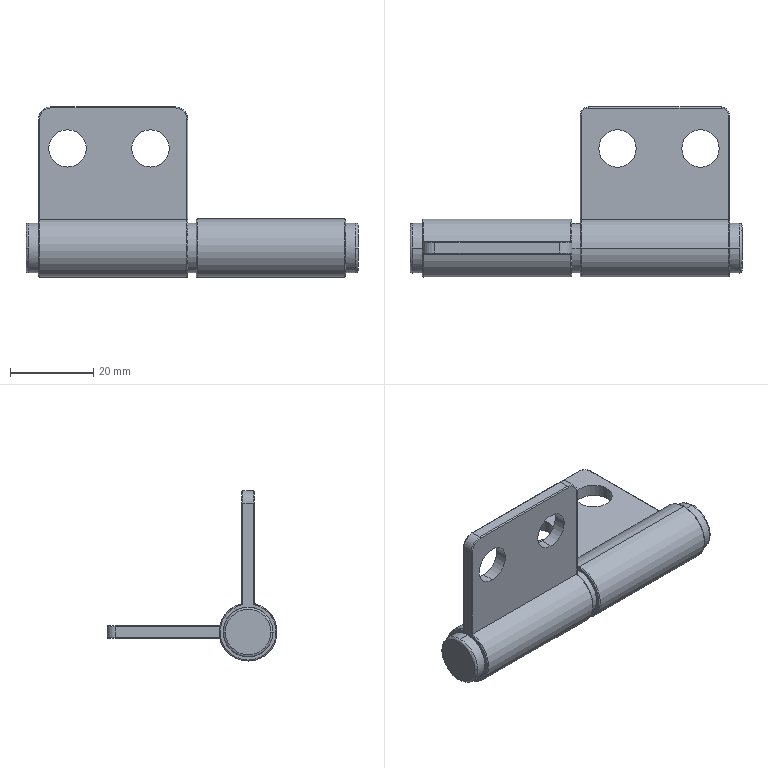Part | STEP file | Instrument cabinet room hinge | 1 solid | 67 faces | box 80 x 41 x 41 mm | volume 17041 mm3 | cylinder 34 | torus 21 | plane 12 | commonest cylinder face diameters 0.5 x12 9 x8 12 x6 14 x4 4 x2 6 x2